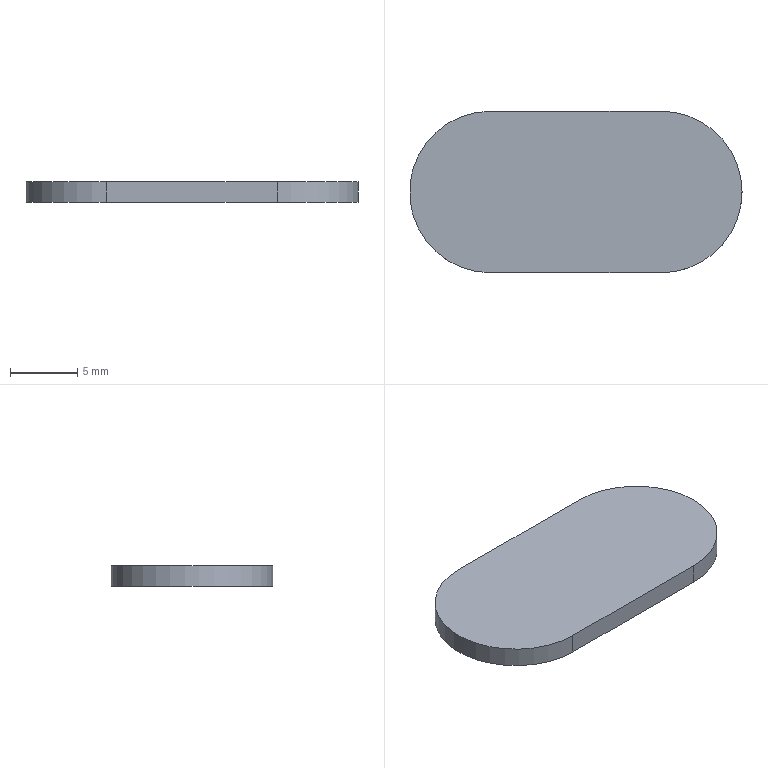Part | STEP file | RS40-AS-2LSR-T-266L-JR-Part-24 | 1 solid | 7 faces | box 24.7 x 12 x 1.5 mm | volume 398.246 mm3 | plane 4 | cylinder 3 | commonest cylinder face diameters 12 x3
STEP:
#1=CARTESIAN_POINT('',(1566.94,2.14,20.9));
#2=VERTEX_POINT('',#1);
#3=CARTESIAN_POINT('',(1560.94,-3.86,20.9));
#4=VERTEX_POINT('',#3);
#5=CARTESIAN_POINT('',(1560.94,2.14,20.9));
#6=DIRECTION('',(0.,0.,-1.));
#7=DIRECTION('',(-1.,0.,0.));
#8=AXIS2_PLACEMENT_3D('',#5,#6,#7);
#9=CIRCLE('',#8,6.);
#10=EDGE_CURVE('',#2,#4,#9,.T.);
#11=ORIENTED_EDGE('',*,*,#10,.F.);
#12=CARTESIAN_POINT('',(1566.94,2.14,22.4));
#13=VERTEX_POINT('',#12);
#14=CARTESIAN_POINT('',(1566.94,2.14,20.9));
#15=DIRECTION('',(0.,0.,1.));
#16=VECTOR('',#15,1000.);
#17=LINE('',#14,#16);
#18=EDGE_CURVE('',#2,#13,#17,.T.);
#19=ORIENTED_EDGE('',*,*,#18,.T.);
#20=CARTESIAN_POINT('',(1560.94,-3.86,22.4));
#21=VERTEX_POINT('',#20);
#22=CARTESIAN_POINT('',(1560.94,2.14,22.4));
#23=DIRECTION('',(0.,0.,-1.));
#24=DIRECTION('',(-1.,0.,0.));
#25=AXIS2_PLACEMENT_3D('',#22,#23,#24);
#26=CIRCLE('',#25,6.);
#27=EDGE_CURVE('',#13,#21,#26,.T.);
#28=ORIENTED_EDGE('',*,*,#27,.T.);
#29=CARTESIAN_POINT('',(1560.94,-3.86,20.9));
#30=DIRECTION('',(0.,0.,1.));
#31=VECTOR('',#30,1000.);
#32=LINE('',#29,#31);
#33=EDGE_CURVE('',#4,#21,#32,.T.);
#34=ORIENTED_EDGE('',*,*,#33,.F.);
#35=EDGE_LOOP('',(#11,#19,#28,#34));
#36=FACE_OUTER_BOUND('',#35,.T.);
#37=CARTESIAN_POINT('',(1560.94,2.14,20.9));
#38=DIRECTION('',(0.,0.,1.));
#39=DIRECTION('',(1.,0.,0.));
#40=AXIS2_PLACEMENT_3D('',#37,#38,#39);
#41=CYLINDRICAL_SURFACE('',#40,6.);
#42=ADVANCED_FACE('',(#36),#41,.T.);
#43=CARTESIAN_POINT('',(1548.24,-3.86,22.4));
#44=VERTEX_POINT('',#43);
#45=CARTESIAN_POINT('',(1560.94,-3.86,22.4));
#46=DIRECTION('',(-1.,0.,0.));
#47=VECTOR('',#46,1000.);
#48=LINE('',#45,#47);
#49=EDGE_CURVE('',#21,#44,#48,.T.);
#50=ORIENTED_EDGE('',*,*,#49,.T.);
#51=CARTESIAN_POINT('',(1548.24,-3.86,20.9));
#52=VERTEX_POINT('',#51);
#53=CARTESIAN_POINT('',(1548.24,-3.86,20.9));
#54=DIRECTION('',(0.,0.,1.));
#55=VECTOR('',#54,1000.);
#56=LINE('',#53,#55);
#57=EDGE_CURVE('',#52,#44,#56,.T.);
#58=ORIENTED_EDGE('',*,*,#57,.F.);
#59=CARTESIAN_POINT('',(1560.94,-3.86,20.9));
#60=DIRECTION('',(-1.,0.,0.));
#61=VECTOR('',#60,1000.);
#62=LINE('',#59,#61);
#63=EDGE_CURVE('',#4,#52,#62,.T.);
#64=ORIENTED_EDGE('',*,*,#63,.F.);
#65=ORIENTED_EDGE('',*,*,#33,.T.);
#66=EDGE_LOOP('',(#50,#58,#64,#65));
#67=FACE_OUTER_BOUND('',#66,.T.);
#68=CARTESIAN_POINT('',(1560.94,-3.86,20.9));
#69=DIRECTION('',(0.,1.,0.));
#70=DIRECTION('',(0.,0.,-1.));
#71=AXIS2_PLACEMENT_3D('',#68,#69,#70);
#72=PLANE('',#71);
#73=ADVANCED_FACE('',(#67),#72,.F.);
#74=CARTESIAN_POINT('',(1548.24,8.14,22.4));
#75=VERTEX_POINT('',#74);
#76=CARTESIAN_POINT('',(1548.24,2.14,22.4));
#77=DIRECTION('',(0.,0.,-1.));
#78=DIRECTION('',(-1.,0.,0.));
#79=AXIS2_PLACEMENT_3D('',#76,#77,#78);
#80=CIRCLE('',#79,6.);
#81=EDGE_CURVE('',#44,#75,#80,.T.);
#82=ORIENTED_EDGE('',*,*,#81,.T.);
#83=CARTESIAN_POINT('',(1548.24,8.14,20.9));
#84=VERTEX_POINT('',#83);
#85=CARTESIAN_POINT('',(1548.24,8.14,20.9));
#86=DIRECTION('',(0.,0.,1.));
#87=VECTOR('',#86,1000.);
#88=LINE('',#85,#87);
#89=EDGE_CURVE('',#84,#75,#88,.T.);
#90=ORIENTED_EDGE('',*,*,#89,.F.);
#91=CARTESIAN_POINT('',(1548.24,2.14,20.9));
#92=DIRECTION('',(0.,0.,-1.));
#93=DIRECTION('',(-1.,0.,0.));
#94=AXIS2_PLACEMENT_3D('',#91,#92,#93);
#95=CIRCLE('',#94,6.);
#96=EDGE_CURVE('',#52,#84,#95,.T.);
#97=ORIENTED_EDGE('',*,*,#96,.F.);
#98=ORIENTED_EDGE('',*,*,#57,.T.);
#99=EDGE_LOOP('',(#82,#90,#97,#98));
#100=FACE_OUTER_BOUND('',#99,.T.);
#101=CARTESIAN_POINT('',(1548.24,2.14,20.9));
#102=DIRECTION('',(0.,0.,1.));
#103=DIRECTION('',(1.,0.,0.));
#104=AXIS2_PLACEMENT_3D('',#101,#102,#103);
#105=CYLINDRICAL_SURFACE('',#104,6.);
#106=ADVANCED_FACE('',(#100),#105,.T.);
#107=CARTESIAN_POINT('',(1560.94,8.14,22.4));
#108=VERTEX_POINT('',#107);
#109=CARTESIAN_POINT('',(1548.24,8.14,22.4));
#110=DIRECTION('',(1.,0.,0.));
#111=VECTOR('',#110,1000.);
#112=LINE('',#109,#111);
#113=EDGE_CURVE('',#75,#108,#112,.T.);
#114=ORIENTED_EDGE('',*,*,#113,.T.);
#115=CARTESIAN_POINT('',(1560.94,8.14,20.9));
#116=VERTEX_POINT('',#115);
#117=CARTESIAN_POINT('',(1560.94,8.14,20.9));
#118=DIRECTION('',(0.,0.,1.));
#119=VECTOR('',#118,1000.);
#120=LINE('',#117,#119);
#121=EDGE_CURVE('',#116,#108,#120,.T.);
#122=ORIENTED_EDGE('',*,*,#121,.F.);
#123=CARTESIAN_POINT('',(1548.24,8.14,20.9));
#124=DIRECTION('',(1.,0.,0.));
#125=VECTOR('',#124,1000.);
#126=LINE('',#123,#125);
#127=EDGE_CURVE('',#84,#116,#126,.T.);
#128=ORIENTED_EDGE('',*,*,#127,.F.);
#129=ORIENTED_EDGE('',*,*,#89,.T.);
#130=EDGE_LOOP('',(#114,#122,#128,#129));
#131=FACE_OUTER_BOUND('',#130,.T.);
#132=CARTESIAN_POINT('',(1548.24,8.14,20.9));
#133=DIRECTION('',(0.,-1.,0.));
#134=DIRECTION('',(0.,0.,1.));
#135=AXIS2_PLACEMENT_3D('',#132,#133,#134);
#136=PLANE('',#135);
#137=ADVANCED_FACE('',(#131),#136,.F.);
#138=ORIENTED_EDGE('',*,*,#18,.F.);
#139=CARTESIAN_POINT('',(1560.94,2.14,20.9));
#140=DIRECTION('',(0.,0.,-1.));
#141=DIRECTION('',(-1.,0.,0.));
#142=AXIS2_PLACEMENT_3D('',#139,#140,#141);
#143=CIRCLE('',#142,6.);
#144=EDGE_CURVE('',#116,#2,#143,.T.);
#145=ORIENTED_EDGE('',*,*,#144,.F.);
#146=ORIENTED_EDGE('',*,*,#121,.T.);
#147=CARTESIAN_POINT('',(1560.94,2.14,22.4));
#148=DIRECTION('',(0.,0.,-1.));
#149=DIRECTION('',(-1.,0.,0.));
#150=AXIS2_PLACEMENT_3D('',#147,#148,#149);
#151=CIRCLE('',#150,6.);
#152=EDGE_CURVE('',#108,#13,#151,.T.);
#153=ORIENTED_EDGE('',*,*,#152,.T.);
#154=EDGE_LOOP('',(#138,#145,#146,#153));
#155=FACE_OUTER_BOUND('',#154,.T.);
#156=CARTESIAN_POINT('',(1560.94,2.14,20.9));
#157=DIRECTION('',(0.,0.,1.));
#158=DIRECTION('',(1.,0.,0.));
#159=AXIS2_PLACEMENT_3D('',#156,#157,#158);
#160=CYLINDRICAL_SURFACE('',#159,6.);
#161=ADVANCED_FACE('',(#155),#160,.T.);
#162=ORIENTED_EDGE('',*,*,#63,.T.);
#163=ORIENTED_EDGE('',*,*,#96,.T.);
#164=ORIENTED_EDGE('',*,*,#127,.T.);
#165=ORIENTED_EDGE('',*,*,#144,.T.);
#166=ORIENTED_EDGE('',*,*,#10,.T.);
#167=EDGE_LOOP('',(#162,#163,#164,#165,#166));
#168=FACE_OUTER_BOUND('',#167,.T.);
#169=CARTESIAN_POINT('',(1548.24,2.14,20.9));
#170=DIRECTION('',(0.,0.,-1.));
#171=DIRECTION('',(-1.,0.,0.));
#172=AXIS2_PLACEMENT_3D('',#169,#170,#171);
#173=PLANE('',#172);
#174=ADVANCED_FACE('',(#168),#173,.T.);
#175=ORIENTED_EDGE('',*,*,#49,.F.);
#176=ORIENTED_EDGE('',*,*,#27,.F.);
#177=ORIENTED_EDGE('',*,*,#152,.F.);
#178=ORIENTED_EDGE('',*,*,#113,.F.);
#179=ORIENTED_EDGE('',*,*,#81,.F.);
#180=EDGE_LOOP('',(#175,#176,#177,#178,#179));
#181=FACE_OUTER_BOUND('',#180,.T.);
#182=CARTESIAN_POINT('',(1548.24,2.14,22.4));
#183=DIRECTION('',(0.,0.,-1.));
#184=DIRECTION('',(-1.,0.,0.));
#185=AXIS2_PLACEMENT_3D('',#182,#183,#184);
#186=PLANE('',#185);
#187=ADVANCED_FACE('',(#181),#186,.F.);
#188=CLOSED_SHELL('',(#42,#73,#106,#137,#161,#174,#187));
#189=MANIFOLD_SOLID_BREP('',#188);
#190=CARTESIAN_POINT('',(0.,0.,0.));
#191=DIRECTION('',(0.,0.,1.));
#192=DIRECTION('',(1.,0.,0.));
#193=AXIS2_PLACEMENT_3D('',#190,#191,#192);
#194=(LENGTH_UNIT()NAMED_UNIT(*)SI_UNIT(.MILLI.,.METRE.));
#195=UNCERTAINTY_MEASURE_WITH_UNIT(LENGTH_MEASURE(0.00001),#194,'','');
#196=(NAMED_UNIT(*)PLANE_ANGLE_UNIT()SI_UNIT($,.RADIAN.));
#197=(NAMED_UNIT(*)SI_UNIT($,.STERADIAN.)SOLID_ANGLE_UNIT());
#198=(GEOMETRIC_REPRESENTATION_CONTEXT(3)GLOBAL_UNCERTAINTY_ASSIGNED_CONTEXT((#195))GLOBAL_UNIT_ASSIGNED_CONTEXT((#194,#196,#197))REPRESENTATION_CONTEXT('',''));
#199=ADVANCED_BREP_SHAPE_REPRESENTATION('',(#189,#193),#198);